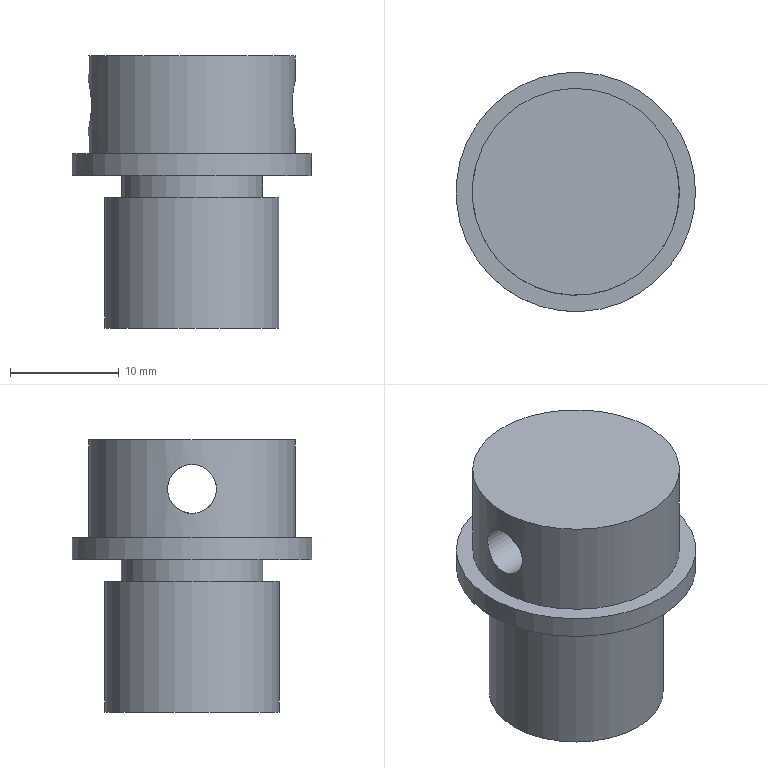Part | NX | features DATUM_CSYS 6, EXTRUDE 5, SKETCH 5 | 1 solid | 10 faces | box 22 x 22 x 25 mm | volume 5690 mm3 | cylinder 5 | plane 5 | commonest cylinder face diameters 4.5 x1 13 x1 16 x1 19 x1 22 x1
STEP:
#1=CARTESIAN_POINT('',(9.5,0.,9.));
#2=VERTEX_POINT('',#1);
#3=CARTESIAN_POINT('',(0.,0.,9.));
#4=DIRECTION('',(0.,0.,1.));
#5=DIRECTION('',(1.,0.,0.));
#6=AXIS2_PLACEMENT_3D('',#3,#4,#5);
#7=CIRCLE('',#6,9.5);
#8=EDGE_CURVE('',#2,#2,#7,.T.);
#9=ORIENTED_EDGE('',*,*,#8,.F.);
#10=EDGE_LOOP('',(#9));
#11=FACE_BOUND('',#10,.T.);
#12=CARTESIAN_POINT('',(9.5,0.,0.));
#13=VERTEX_POINT('',#12);
#14=CARTESIAN_POINT('',(0.,0.,0.));
#15=DIRECTION('',(0.,0.,1.));
#16=DIRECTION('',(1.,0.,0.));
#17=AXIS2_PLACEMENT_3D('',#14,#15,#16);
#18=CIRCLE('',#17,9.5);
#19=EDGE_CURVE('',#13,#13,#18,.T.);
#20=ORIENTED_EDGE('',*,*,#19,.T.);
#21=EDGE_LOOP('',(#20));
#22=FACE_BOUND('',#21,.T.);
#23=CARTESIAN_POINT('',(9.5,0.,6.75));
#24=VERTEX_POINT('',#23);
#25=CARTESIAN_POINT('',(9.366,1.765,6.262));
#26=CARTESIAN_POINT('',(9.567,-0.0003471,6.994));
#27=CARTESIAN_POINT('',(9.367,-1.764,6.262));
#28=CARTESIAN_POINT('',(9.161,-2.493,4.503));
#29=CARTESIAN_POINT('',(9.367,-1.763,2.736));
#30=CARTESIAN_POINT('',(9.567,-0.0009977,2.007));
#31=CARTESIAN_POINT('',(9.367,1.762,2.735));
#32=CARTESIAN_POINT('',(9.161,2.493,4.499));
#33=CARTESIAN_POINT('',(9.366,1.765,6.262));
#34=CARTESIAN_POINT('',(9.567,-0.0003471,6.994));
#35=CARTESIAN_POINT('',(9.367,-1.764,6.262));
#36=B_SPLINE_CURVE_WITH_KNOTS('',3,(#25,#26,#27,#28,#29,#30,#31,#32,#33,#34,#35),.UNSPECIFIED.,.T.,.F.,(1,1,1,1,1,1,1,1,1,1,1,1,1,1,1),(-0.005294,-0.003529,-0.001765,0.,0.001765,0.003529,0.005294,0.007059,0.008823,0.01059,0.01235,0.01412,0.01588,0.01765,0.01941),.UNSPECIFIED.);
#37=EDGE_CURVE('',#24,#24,#36,.T.);
#38=ORIENTED_EDGE('',*,*,#37,.F.);
#39=EDGE_LOOP('',(#38));
#40=FACE_BOUND('',#39,.T.);
#41=CARTESIAN_POINT('',(-9.5,0.,6.75));
#42=VERTEX_POINT('',#41);
#43=CARTESIAN_POINT('',(-9.366,-1.765,6.262));
#44=CARTESIAN_POINT('',(-9.567,0.0003471,6.994));
#45=CARTESIAN_POINT('',(-9.367,1.764,6.262));
#46=CARTESIAN_POINT('',(-9.161,2.493,4.503));
#47=CARTESIAN_POINT('',(-9.367,1.763,2.736));
#48=CARTESIAN_POINT('',(-9.567,0.0009977,2.007));
#49=CARTESIAN_POINT('',(-9.367,-1.762,2.735));
#50=CARTESIAN_POINT('',(-9.161,-2.493,4.499));
#51=CARTESIAN_POINT('',(-9.366,-1.765,6.262));
#52=CARTESIAN_POINT('',(-9.567,0.0003471,6.994));
#53=CARTESIAN_POINT('',(-9.367,1.764,6.262));
#54=B_SPLINE_CURVE_WITH_KNOTS('',3,(#43,#44,#45,#46,#47,#48,#49,#50,#51,#52,#53),.UNSPECIFIED.,.T.,.F.,(1,1,1,1,1,1,1,1,1,1,1,1,1,1,1),(-0.005294,-0.003529,-0.001765,0.,0.001765,0.003529,0.005294,0.007059,0.008823,0.01059,0.01235,0.01412,0.01588,0.01765,0.01941),.UNSPECIFIED.);
#55=EDGE_CURVE('',#42,#42,#54,.T.);
#56=ORIENTED_EDGE('',*,*,#55,.F.);
#57=EDGE_LOOP('',(#56));
#58=FACE_BOUND('',#57,.T.);
#59=CARTESIAN_POINT('',(0.,0.,9.));
#60=DIRECTION('',(0.,0.,-1.));
#61=DIRECTION('',(-1.,0.,0.));
#62=AXIS2_PLACEMENT_3D('',#59,#60,#61);
#63=CYLINDRICAL_SURFACE('',#62,9.5);
#64=ADVANCED_FACE('',(#11,#22,#40,#58),#63,.T.);
#65=ORIENTED_EDGE('',*,*,#8,.T.);
#66=EDGE_LOOP('',(#65));
#67=FACE_BOUND('',#66,.T.);
#68=CARTESIAN_POINT('',(0.,0.,9.));
#69=DIRECTION('',(0.,0.,1.));
#70=DIRECTION('',(1.,0.,0.));
#71=AXIS2_PLACEMENT_3D('',#68,#69,#70);
#72=PLANE('',#71);
#73=ADVANCED_FACE('',(#67),#72,.T.);
#74=CARTESIAN_POINT('',(11.,0.,-2.));
#75=VERTEX_POINT('',#74);
#76=CARTESIAN_POINT('',(0.,0.,-2.));
#77=DIRECTION('',(0.,0.,-1.));
#78=DIRECTION('',(1.,0.,0.));
#79=AXIS2_PLACEMENT_3D('',#76,#77,#78);
#80=CIRCLE('',#79,11.);
#81=EDGE_CURVE('',#75,#75,#80,.T.);
#82=ORIENTED_EDGE('',*,*,#81,.F.);
#83=EDGE_LOOP('',(#82));
#84=FACE_BOUND('',#83,.T.);
#85=CARTESIAN_POINT('',(11.,0.,0.));
#86=VERTEX_POINT('',#85);
#87=CARTESIAN_POINT('',(0.,0.,0.));
#88=DIRECTION('',(0.,0.,-1.));
#89=DIRECTION('',(1.,0.,0.));
#90=AXIS2_PLACEMENT_3D('',#87,#88,#89);
#91=CIRCLE('',#90,11.);
#92=EDGE_CURVE('',#86,#86,#91,.T.);
#93=ORIENTED_EDGE('',*,*,#92,.T.);
#94=EDGE_LOOP('',(#93));
#95=FACE_BOUND('',#94,.T.);
#96=CARTESIAN_POINT('',(0.,0.,-2.));
#97=DIRECTION('',(0.,0.,1.));
#98=DIRECTION('',(1.,0.,0.));
#99=AXIS2_PLACEMENT_3D('',#96,#97,#98);
#100=CYLINDRICAL_SURFACE('',#99,11.);
#101=ADVANCED_FACE('',(#84,#95),#100,.T.);
#102=CARTESIAN_POINT('',(6.5,0.,-2.));
#103=VERTEX_POINT('',#102);
#104=CARTESIAN_POINT('',(0.,0.,-2.));
#105=DIRECTION('',(0.,0.,-1.));
#106=DIRECTION('',(1.,0.,0.));
#107=AXIS2_PLACEMENT_3D('',#104,#105,#106);
#108=CIRCLE('',#107,6.5);
#109=EDGE_CURVE('',#103,#103,#108,.T.);
#110=ORIENTED_EDGE('',*,*,#109,.F.);
#111=EDGE_LOOP('',(#110));
#112=FACE_BOUND('',#111,.T.);
#113=ORIENTED_EDGE('',*,*,#81,.T.);
#114=EDGE_LOOP('',(#113));
#115=FACE_BOUND('',#114,.T.);
#116=CARTESIAN_POINT('',(0.,0.,-2.));
#117=DIRECTION('',(0.,0.,-1.));
#118=DIRECTION('',(-1.,0.,0.));
#119=AXIS2_PLACEMENT_3D('',#116,#117,#118);
#120=PLANE('',#119);
#121=ADVANCED_FACE('',(#112,#115),#120,.T.);
#122=ORIENTED_EDGE('',*,*,#19,.F.);
#123=EDGE_LOOP('',(#122));
#124=FACE_BOUND('',#123,.T.);
#125=ORIENTED_EDGE('',*,*,#92,.F.);
#126=EDGE_LOOP('',(#125));
#127=FACE_BOUND('',#126,.T.);
#128=CARTESIAN_POINT('',(0.,0.,0.));
#129=DIRECTION('',(0.,0.,-1.));
#130=DIRECTION('',(-1.,0.,0.));
#131=AXIS2_PLACEMENT_3D('',#128,#129,#130);
#132=PLANE('',#131);
#133=ADVANCED_FACE('',(#124,#127),#132,.F.);
#134=CARTESIAN_POINT('',(6.5,0.,-4.));
#135=VERTEX_POINT('',#134);
#136=CARTESIAN_POINT('',(0.,0.,-4.));
#137=DIRECTION('',(0.,0.,-1.));
#138=DIRECTION('',(1.,0.,0.));
#139=AXIS2_PLACEMENT_3D('',#136,#137,#138);
#140=CIRCLE('',#139,6.5);
#141=EDGE_CURVE('',#135,#135,#140,.T.);
#142=ORIENTED_EDGE('',*,*,#141,.F.);
#143=EDGE_LOOP('',(#142));
#144=FACE_BOUND('',#143,.T.);
#145=ORIENTED_EDGE('',*,*,#109,.T.);
#146=EDGE_LOOP('',(#145));
#147=FACE_BOUND('',#146,.T.);
#148=CARTESIAN_POINT('',(0.,0.,-4.));
#149=DIRECTION('',(0.,0.,1.));
#150=DIRECTION('',(1.,0.,0.));
#151=AXIS2_PLACEMENT_3D('',#148,#149,#150);
#152=CYLINDRICAL_SURFACE('',#151,6.5);
#153=ADVANCED_FACE('',(#144,#147),#152,.T.);
#154=CARTESIAN_POINT('',(8.,0.,-16.));
#155=VERTEX_POINT('',#154);
#156=CARTESIAN_POINT('',(0.,0.,-16.));
#157=DIRECTION('',(0.,0.,-1.));
#158=DIRECTION('',(1.,0.,0.));
#159=AXIS2_PLACEMENT_3D('',#156,#157,#158);
#160=CIRCLE('',#159,8.);
#161=EDGE_CURVE('',#155,#155,#160,.T.);
#162=ORIENTED_EDGE('',*,*,#161,.F.);
#163=EDGE_LOOP('',(#162));
#164=FACE_BOUND('',#163,.T.);
#165=CARTESIAN_POINT('',(8.,0.,-4.));
#166=VERTEX_POINT('',#165);
#167=CARTESIAN_POINT('',(0.,0.,-4.));
#168=DIRECTION('',(0.,0.,-1.));
#169=DIRECTION('',(1.,0.,0.));
#170=AXIS2_PLACEMENT_3D('',#167,#168,#169);
#171=CIRCLE('',#170,8.);
#172=EDGE_CURVE('',#166,#166,#171,.T.);
#173=ORIENTED_EDGE('',*,*,#172,.T.);
#174=EDGE_LOOP('',(#173));
#175=FACE_BOUND('',#174,.T.);
#176=CARTESIAN_POINT('',(0.,0.,-16.));
#177=DIRECTION('',(0.,0.,1.));
#178=DIRECTION('',(1.,0.,0.));
#179=AXIS2_PLACEMENT_3D('',#176,#177,#178);
#180=CYLINDRICAL_SURFACE('',#179,8.);
#181=ADVANCED_FACE('',(#164,#175),#180,.T.);
#182=ORIENTED_EDGE('',*,*,#161,.T.);
#183=EDGE_LOOP('',(#182));
#184=FACE_BOUND('',#183,.T.);
#185=CARTESIAN_POINT('',(0.,0.,-16.));
#186=DIRECTION('',(0.,0.,-1.));
#187=DIRECTION('',(-1.,0.,0.));
#188=AXIS2_PLACEMENT_3D('',#185,#186,#187);
#189=PLANE('',#188);
#190=ADVANCED_FACE('',(#184),#189,.T.);
#191=ORIENTED_EDGE('',*,*,#141,.T.);
#192=EDGE_LOOP('',(#191));
#193=FACE_BOUND('',#192,.T.);
#194=ORIENTED_EDGE('',*,*,#172,.F.);
#195=EDGE_LOOP('',(#194));
#196=FACE_BOUND('',#195,.T.);
#197=CARTESIAN_POINT('',(0.,0.,-4.));
#198=DIRECTION('',(0.,0.,-1.));
#199=DIRECTION('',(-1.,0.,0.));
#200=AXIS2_PLACEMENT_3D('',#197,#198,#199);
#201=PLANE('',#200);
#202=ADVANCED_FACE('',(#193,#196),#201,.F.);
#203=ORIENTED_EDGE('',*,*,#37,.T.);
#204=EDGE_LOOP('',(#203));
#205=FACE_BOUND('',#204,.T.);
#206=ORIENTED_EDGE('',*,*,#55,.T.);
#207=EDGE_LOOP('',(#206));
#208=FACE_BOUND('',#207,.T.);
#209=CARTESIAN_POINT('',(18.,0.,4.5));
#210=DIRECTION('',(-1.,0.,0.));
#211=DIRECTION('',(0.,0.,1.));
#212=AXIS2_PLACEMENT_3D('',#209,#210,#211);
#213=CYLINDRICAL_SURFACE('',#212,2.25);
#214=ADVANCED_FACE('',(#205,#208),#213,.F.);
#215=CLOSED_SHELL('',(#64,#73,#101,#121,#133,#153,#181,#190,#202,#214));
#216=MANIFOLD_SOLID_BREP('',#215);
#217=(LENGTH_UNIT()NAMED_UNIT(*)SI_UNIT(.MILLI.,.METRE.));
#218=UNCERTAINTY_MEASURE_WITH_UNIT(LENGTH_MEASURE(0.0508),#217,'','');
#219=(NAMED_UNIT(*)PLANE_ANGLE_UNIT()SI_UNIT($,.RADIAN.));
#220=(NAMED_UNIT(*)SI_UNIT($,.STERADIAN.)SOLID_ANGLE_UNIT());
#221=(GEOMETRIC_REPRESENTATION_CONTEXT(3)GLOBAL_UNCERTAINTY_ASSIGNED_CONTEXT((#218))GLOBAL_UNIT_ASSIGNED_CONTEXT((#217,#219,#220))REPRESENTATION_CONTEXT('',''));
#222=ADVANCED_BREP_SHAPE_REPRESENTATION('',(#216),#221);